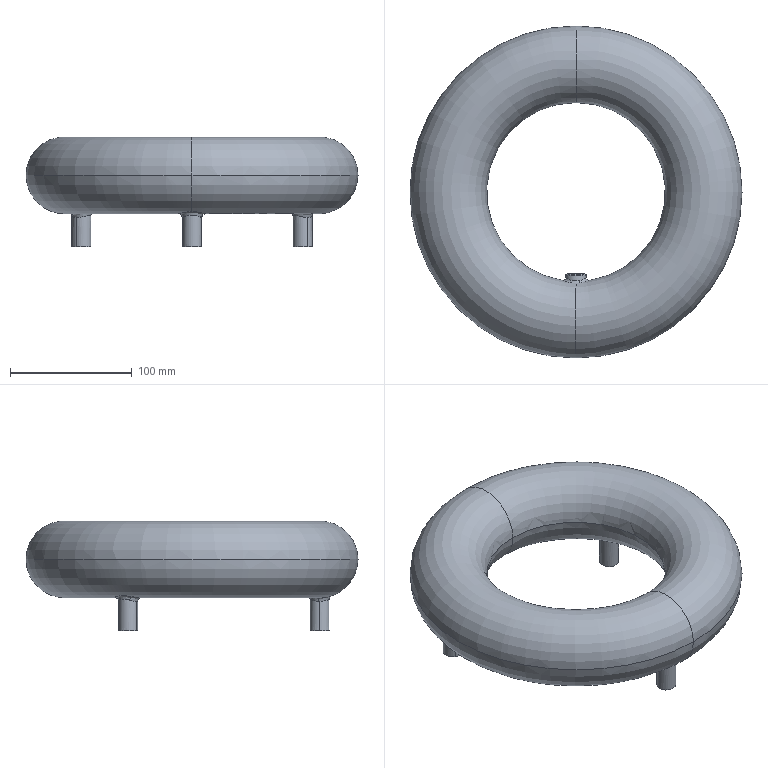Part | SolidWorks | features Fillet 4, BaseBody 1, ICE 1, Scale 1 | 1 solid | 48 faces | box 273 x 273 x 90.3 mm | volume 274529 mm3 | torus 16 | cylinder 16 | spline 10 | plane 4 | cone 2 | commonest cylinder face diameters 10.5 x6 15.75 x6 12.6 x2 16.8 x2